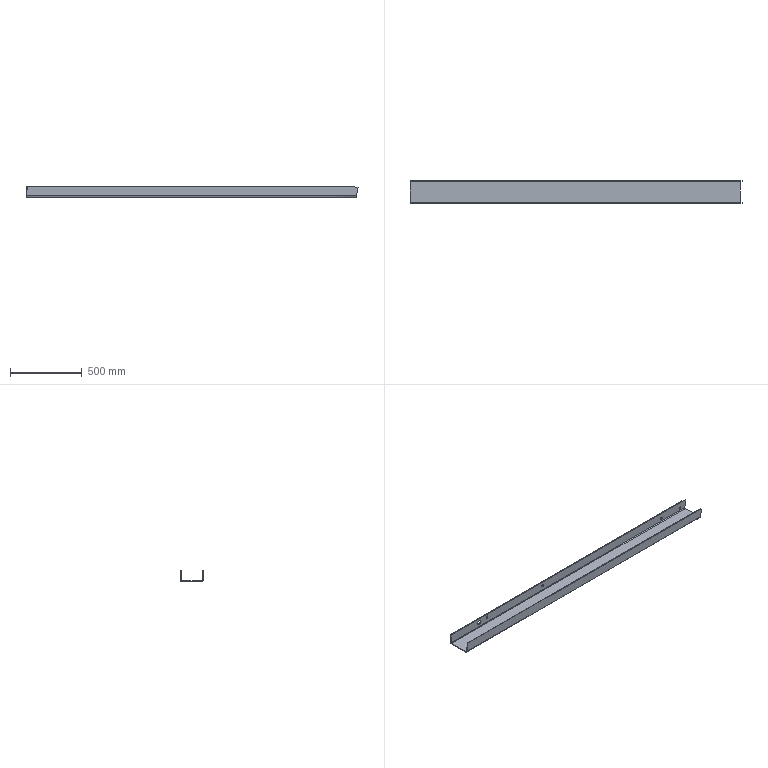Part | SolidWorks | features Split 4, Cut 2, 3DProfileFeature 1, FlatPattern 1, Fold 1, HoleWzd 1, SM3dBend 1, SMBaseFlange 1, SheetMetal 1, UnFold 1, WeldmentFeature 1 | 1 solid | 35 faces | box 2311 x 160 x 74.999 mm | volume 3368982 mm3 | plane 18 | cylinder 14 | spline 3 | commonest cylinder face diameters 18 x8 10 x2 20 x2 30 x2
STEP:
#1=CARTESIAN_POINT('',(-396.279,75.,50.082));
#2=VERTEX_POINT('',#1);
#3=CARTESIAN_POINT('',(-396.279,75.,32.082));
#4=VERTEX_POINT('',#3);
#5=CARTESIAN_POINT('',(-396.279,75.,41.082));
#6=DIRECTION('',(0.,-1.,0.));
#7=DIRECTION('',(0.,0.,-1.));
#8=AXIS2_PLACEMENT_3D('',#5,#6,#7);
#9=CIRCLE('',#8,9.);
#10=EDGE_CURVE('',#2,#4,#9,.T.);
#11=ORIENTED_EDGE('',*,*,#10,.T.);
#12=CARTESIAN_POINT('',(-396.279,80.,32.082));
#13=VERTEX_POINT('',#12);
#14=CARTESIAN_POINT('',(-396.279,80.,32.082));
#15=DIRECTION('',(0.,1.,0.));
#16=VECTOR('',#15,1000.);
#17=LINE('',#14,#16);
#18=EDGE_CURVE('',#4,#13,#17,.T.);
#19=ORIENTED_EDGE('',*,*,#18,.T.);
#20=CARTESIAN_POINT('',(-396.279,80.,50.082));
#21=VERTEX_POINT('',#20);
#22=CARTESIAN_POINT('',(-396.279,80.,41.082));
#23=DIRECTION('',(0.,1.,0.));
#24=DIRECTION('',(0.,0.,1.));
#25=AXIS2_PLACEMENT_3D('',#22,#23,#24);
#26=CIRCLE('',#25,9.);
#27=EDGE_CURVE('',#13,#21,#26,.T.);
#28=ORIENTED_EDGE('',*,*,#27,.T.);
#29=CARTESIAN_POINT('',(-396.279,80.,50.082));
#30=DIRECTION('',(0.,1.,0.));
#31=VECTOR('',#30,1000.);
#32=LINE('',#29,#31);
#33=EDGE_CURVE('',#2,#21,#32,.T.);
#34=ORIENTED_EDGE('',*,*,#33,.F.);
#35=EDGE_LOOP('',(#11,#19,#28,#34));
#36=FACE_OUTER_BOUND('',#35,.T.);
#37=CARTESIAN_POINT('',(-396.279,80.,41.082));
#38=DIRECTION('',(0.,1.,0.));
#39=DIRECTION('',(0.,0.,1.));
#40=AXIS2_PLACEMENT_3D('',#37,#38,#39);
#41=CYLINDRICAL_SURFACE('',#40,9.);
#42=ADVANCED_FACE('',(#36),#41,.F.);
#43=CARTESIAN_POINT('',(-945.843,75.,53.474));
#44=VERTEX_POINT('',#43);
#45=CARTESIAN_POINT('',(-945.843,75.,35.474));
#46=VERTEX_POINT('',#45);
#47=CARTESIAN_POINT('',(-945.843,75.,44.474));
#48=DIRECTION('',(0.,-1.,0.));
#49=DIRECTION('',(0.,0.,-1.));
#50=AXIS2_PLACEMENT_3D('',#47,#48,#49);
#51=CIRCLE('',#50,9.);
#52=EDGE_CURVE('',#44,#46,#51,.T.);
#53=ORIENTED_EDGE('',*,*,#52,.T.);
#54=CARTESIAN_POINT('',(-945.843,80.,35.474));
#55=VERTEX_POINT('',#54);
#56=CARTESIAN_POINT('',(-945.843,80.,35.474));
#57=DIRECTION('',(0.,1.,0.));
#58=VECTOR('',#57,1000.);
#59=LINE('',#56,#58);
#60=EDGE_CURVE('',#46,#55,#59,.T.);
#61=ORIENTED_EDGE('',*,*,#60,.T.);
#62=CARTESIAN_POINT('',(-945.843,80.,53.474));
#63=VERTEX_POINT('',#62);
#64=CARTESIAN_POINT('',(-945.843,80.,44.474));
#65=DIRECTION('',(0.,1.,0.));
#66=DIRECTION('',(0.,0.,1.));
#67=AXIS2_PLACEMENT_3D('',#64,#65,#66);
#68=CIRCLE('',#67,9.);
#69=EDGE_CURVE('',#55,#63,#68,.T.);
#70=ORIENTED_EDGE('',*,*,#69,.T.);
#71=CARTESIAN_POINT('',(-945.843,80.,53.474));
#72=DIRECTION('',(0.,1.,0.));
#73=VECTOR('',#72,1000.);
#74=LINE('',#71,#73);
#75=EDGE_CURVE('',#44,#63,#74,.T.);
#76=ORIENTED_EDGE('',*,*,#75,.F.);
#77=EDGE_LOOP('',(#53,#61,#70,#76));
#78=FACE_OUTER_BOUND('',#77,.T.);
#79=CARTESIAN_POINT('',(-945.843,80.,44.474));
#80=DIRECTION('',(0.,1.,0.));
#81=DIRECTION('',(0.,0.,1.));
#82=AXIS2_PLACEMENT_3D('',#79,#80,#81);
#83=CYLINDRICAL_SURFACE('',#82,9.);
#84=ADVANCED_FACE('',(#78),#83,.F.);
#85=CARTESIAN_POINT('',(772.235,75.,37.443));
#86=VERTEX_POINT('',#85);
#87=CARTESIAN_POINT('',(772.235,75.,19.443));
#88=VERTEX_POINT('',#87);
#89=CARTESIAN_POINT('',(772.235,75.,28.443));
#90=DIRECTION('',(0.,-1.,0.));
#91=DIRECTION('',(0.,0.,-1.));
#92=AXIS2_PLACEMENT_3D('',#89,#90,#91);
#93=CIRCLE('',#92,9.);
#94=EDGE_CURVE('',#86,#88,#93,.T.);
#95=ORIENTED_EDGE('',*,*,#94,.T.);
#96=CARTESIAN_POINT('',(772.235,80.,19.443));
#97=VERTEX_POINT('',#96);
#98=CARTESIAN_POINT('',(772.235,70.,19.443));
#99=DIRECTION('',(0.,1.,0.));
#100=VECTOR('',#99,1000.);
#101=LINE('',#98,#100);
#102=EDGE_CURVE('',#88,#97,#101,.T.);
#103=ORIENTED_EDGE('',*,*,#102,.T.);
#104=CARTESIAN_POINT('',(772.235,80.,37.443));
#105=VERTEX_POINT('',#104);
#106=CARTESIAN_POINT('',(772.235,80.,28.443));
#107=DIRECTION('',(0.,1.,0.));
#108=DIRECTION('',(0.,0.,1.));
#109=AXIS2_PLACEMENT_3D('',#106,#107,#108);
#110=CIRCLE('',#109,9.);
#111=EDGE_CURVE('',#97,#105,#110,.T.);
#112=ORIENTED_EDGE('',*,*,#111,.T.);
#113=CARTESIAN_POINT('',(772.235,70.,37.443));
#114=DIRECTION('',(0.,1.,0.));
#115=VECTOR('',#114,1000.);
#116=LINE('',#113,#115);
#117=EDGE_CURVE('',#86,#105,#116,.T.);
#118=ORIENTED_EDGE('',*,*,#117,.F.);
#119=EDGE_LOOP('',(#95,#103,#112,#118));
#120=FACE_OUTER_BOUND('',#119,.T.);
#121=CARTESIAN_POINT('',(772.235,70.,28.443));
#122=DIRECTION('',(0.,1.,0.));
#123=DIRECTION('',(0.,0.,1.));
#124=AXIS2_PLACEMENT_3D('',#121,#122,#123);
#125=CYLINDRICAL_SURFACE('',#124,9.);
#126=ADVANCED_FACE('',(#120),#125,.F.);
#127=CARTESIAN_POINT('',(953.893,75.,32.391));
#128=VERTEX_POINT('',#127);
#129=CARTESIAN_POINT('',(953.893,75.,14.391));
#130=VERTEX_POINT('',#129);
#131=CARTESIAN_POINT('',(953.893,75.,23.391));
#132=DIRECTION('',(0.,-1.,0.));
#133=DIRECTION('',(0.,0.,-1.));
#134=AXIS2_PLACEMENT_3D('',#131,#132,#133);
#135=CIRCLE('',#134,9.);
#136=EDGE_CURVE('',#128,#130,#135,.T.);
#137=ORIENTED_EDGE('',*,*,#136,.T.);
#138=CARTESIAN_POINT('',(953.893,80.,14.391));
#139=VERTEX_POINT('',#138);
#140=CARTESIAN_POINT('',(953.893,70.,14.391));
#141=DIRECTION('',(0.,1.,0.));
#142=VECTOR('',#141,1000.);
#143=LINE('',#140,#142);
#144=EDGE_CURVE('',#130,#139,#143,.T.);
#145=ORIENTED_EDGE('',*,*,#144,.T.);
#146=CARTESIAN_POINT('',(953.893,80.,32.391));
#147=VERTEX_POINT('',#146);
#148=CARTESIAN_POINT('',(953.893,80.,23.391));
#149=DIRECTION('',(0.,1.,0.));
#150=DIRECTION('',(0.,0.,1.));
#151=AXIS2_PLACEMENT_3D('',#148,#149,#150);
#152=CIRCLE('',#151,9.);
#153=EDGE_CURVE('',#139,#147,#152,.T.);
#154=ORIENTED_EDGE('',*,*,#153,.T.);
#155=CARTESIAN_POINT('',(953.893,70.,32.391));
#156=DIRECTION('',(0.,1.,0.));
#157=VECTOR('',#156,1000.);
#158=LINE('',#155,#157);
#159=EDGE_CURVE('',#128,#147,#158,.T.);
#160=ORIENTED_EDGE('',*,*,#159,.F.);
#161=EDGE_LOOP('',(#137,#145,#154,#160));
#162=FACE_OUTER_BOUND('',#161,.T.);
#163=CARTESIAN_POINT('',(953.893,70.,23.391));
#164=DIRECTION('',(0.,1.,0.));
#165=DIRECTION('',(0.,0.,1.));
#166=AXIS2_PLACEMENT_3D('',#163,#164,#165);
#167=CYLINDRICAL_SURFACE('',#166,9.);
#168=ADVANCED_FACE('',(#162),#167,.F.);
#169=CARTESIAN_POINT('',(-1024.117,75.,52.057));
#170=VERTEX_POINT('',#169);
#171=CARTESIAN_POINT('',(-1024.117,75.,22.057));
#172=VERTEX_POINT('',#171);
#173=CARTESIAN_POINT('',(-1024.117,75.,37.057));
#174=DIRECTION('',(0.,-1.,0.));
#175=DIRECTION('',(0.,0.,-1.));
#176=AXIS2_PLACEMENT_3D('',#173,#174,#175);
#177=CIRCLE('',#176,15.);
#178=EDGE_CURVE('',#170,#172,#177,.T.);
#179=ORIENTED_EDGE('',*,*,#178,.T.);
#180=CARTESIAN_POINT('',(-1024.117,80.,22.057));
#181=VERTEX_POINT('',#180);
#182=CARTESIAN_POINT('',(-1024.117,70.,22.057));
#183=DIRECTION('',(0.,1.,0.));
#184=VECTOR('',#183,1000.);
#185=LINE('',#182,#184);
#186=EDGE_CURVE('',#172,#181,#185,.T.);
#187=ORIENTED_EDGE('',*,*,#186,.T.);
#188=CARTESIAN_POINT('',(-1024.117,80.,52.057));
#189=VERTEX_POINT('',#188);
#190=CARTESIAN_POINT('',(-1024.117,80.,37.057));
#191=DIRECTION('',(0.,1.,0.));
#192=DIRECTION('',(0.,0.,1.));
#193=AXIS2_PLACEMENT_3D('',#190,#191,#192);
#194=CIRCLE('',#193,15.);
#195=EDGE_CURVE('',#181,#189,#194,.T.);
#196=ORIENTED_EDGE('',*,*,#195,.T.);
#197=CARTESIAN_POINT('',(-1024.117,70.,52.057));
#198=DIRECTION('',(0.,1.,0.));
#199=VECTOR('',#198,1000.);
#200=LINE('',#197,#199);
#201=EDGE_CURVE('',#170,#189,#200,.T.);
#202=ORIENTED_EDGE('',*,*,#201,.F.);
#203=EDGE_LOOP('',(#179,#187,#196,#202));
#204=FACE_OUTER_BOUND('',#203,.T.);
#205=CARTESIAN_POINT('',(-1024.117,70.,37.057));
#206=DIRECTION('',(0.,1.,0.));
#207=DIRECTION('',(0.,0.,1.));
#208=AXIS2_PLACEMENT_3D('',#205,#206,#207);
#209=CYLINDRICAL_SURFACE('',#208,15.);
#210=ADVANCED_FACE('',(#204),#209,.F.);
#211=CARTESIAN_POINT('',(-945.843,80.,44.474));
#212=DIRECTION('',(0.,1.,0.));
#213=DIRECTION('',(0.,0.,1.));
#214=AXIS2_PLACEMENT_3D('',#211,#212,#213);
#215=CIRCLE('',#214,9.);
#216=EDGE_CURVE('',#63,#55,#215,.T.);
#217=ORIENTED_EDGE('',*,*,#216,.F.);
#218=ORIENTED_EDGE('',*,*,#69,.F.);
#219=EDGE_LOOP('',(#217,#218));
#220=FACE_BOUND('',#219,.T.);
#221=CARTESIAN_POINT('',(772.235,80.,28.443));
#222=DIRECTION('',(0.,1.,0.));
#223=DIRECTION('',(0.,0.,1.));
#224=AXIS2_PLACEMENT_3D('',#221,#222,#223);
#225=CIRCLE('',#224,9.);
#226=EDGE_CURVE('',#105,#97,#225,.T.);
#227=ORIENTED_EDGE('',*,*,#226,.F.);
#228=ORIENTED_EDGE('',*,*,#111,.F.);
#229=EDGE_LOOP('',(#227,#228));
#230=FACE_BOUND('',#229,.T.);
#231=CARTESIAN_POINT('',(953.893,80.,23.391));
#232=DIRECTION('',(0.,1.,0.));
#233=DIRECTION('',(0.,0.,1.));
#234=AXIS2_PLACEMENT_3D('',#231,#232,#233);
#235=CIRCLE('',#234,9.);
#236=EDGE_CURVE('',#147,#139,#235,.T.);
#237=ORIENTED_EDGE('',*,*,#236,.F.);
#238=ORIENTED_EDGE('',*,*,#153,.F.);
#239=EDGE_LOOP('',(#237,#238));
#240=FACE_BOUND('',#239,.T.);
#241=CARTESIAN_POINT('',(-1024.117,80.,37.057));
#242=DIRECTION('',(0.,1.,0.));
#243=DIRECTION('',(0.,0.,1.));
#244=AXIS2_PLACEMENT_3D('',#241,#242,#243);
#245=CIRCLE('',#244,15.);
#246=EDGE_CURVE('',#189,#181,#245,.T.);
#247=ORIENTED_EDGE('',*,*,#246,.F.);
#248=ORIENTED_EDGE('',*,*,#195,.F.);
#249=EDGE_LOOP('',(#247,#248));
#250=FACE_BOUND('',#249,.T.);
#251=CARTESIAN_POINT('',(-1299.9,80.,69.999));
#252=VERTEX_POINT('',#251);
#253=CARTESIAN_POINT('',(-1299.9,80.,5.));
#254=VERTEX_POINT('',#253);
#255=CARTESIAN_POINT('',(-1299.9,80.,-76.781));
#256=DIRECTION('',(0.,0.,-1.));
#257=VECTOR('',#256,1000.);
#258=LINE('',#255,#257);
#259=EDGE_CURVE('',#252,#254,#258,.T.);
#260=ORIENTED_EDGE('',*,*,#259,.F.);
#261=CARTESIAN_POINT('',(978.319,80.,69.999));
#262=VERTEX_POINT('',#261);
#263=CARTESIAN_POINT('',(-1300.,80.,69.999));
#264=DIRECTION('',(-1.,0.,0.));
#265=VECTOR('',#264,1000.);
#266=LINE('',#263,#265);
#267=EDGE_CURVE('',#262,#252,#266,.T.);
#268=ORIENTED_EDGE('',*,*,#267,.F.);
#269=CARTESIAN_POINT('',(1011.459,80.,64.453));
#270=VERTEX_POINT('',#269);
#271=CARTESIAN_POINT('',(50.544,80.,225.255));
#272=DIRECTION('',(-0.9863,0.,0.165));
#273=VECTOR('',#272,1000.);
#274=LINE('',#271,#273);
#275=EDGE_CURVE('',#270,#262,#274,.T.);
#276=ORIENTED_EDGE('',*,*,#275,.F.);
#277=CARTESIAN_POINT('',(1001.51,80.,5.));
#278=VERTEX_POINT('',#277);
#279=CARTESIAN_POINT('',(960.916,80.,-237.583));
#280=DIRECTION('',(-0.165,0.,-0.9863));
#281=VECTOR('',#280,1000.);
#282=LINE('',#279,#281);
#283=EDGE_CURVE('',#270,#278,#282,.T.);
#284=ORIENTED_EDGE('',*,*,#283,.T.);
#285=CARTESIAN_POINT('',(-1299.9,80.,5.));
#286=CARTESIAN_POINT('',(-532.763,80.,5.));
#287=CARTESIAN_POINT('',(234.373,80.,5.));
#288=CARTESIAN_POINT('',(1001.51,80.,5.));
#289=B_SPLINE_CURVE_WITH_KNOTS('',3,(#285,#286,#287,#288),.UNSPECIFIED.,.F.,.F.,(4,4),(0.,1.),.UNSPECIFIED.);
#290=EDGE_CURVE('',#254,#278,#289,.T.);
#291=ORIENTED_EDGE('',*,*,#290,.F.);
#292=EDGE_LOOP('',(#260,#268,#276,#284,#291));
#293=FACE_OUTER_BOUND('',#292,.T.);
#294=CARTESIAN_POINT('',(-396.279,80.,41.082));
#295=DIRECTION('',(0.,1.,0.));
#296=DIRECTION('',(0.,0.,1.));
#297=AXIS2_PLACEMENT_3D('',#294,#295,#296);
#298=CIRCLE('',#297,9.);
#299=EDGE_CURVE('',#21,#13,#298,.T.);
#300=ORIENTED_EDGE('',*,*,#299,.F.);
#301=ORIENTED_EDGE('',*,*,#27,.F.);
#302=EDGE_LOOP('',(#300,#301));
#303=FACE_BOUND('',#302,.T.);
#304=CARTESIAN_POINT('',(0.,80.,-76.781));
#305=DIRECTION('',(0.,-1.,0.));
#306=DIRECTION('',(1.,0.,0.));
#307=AXIS2_PLACEMENT_3D('',#304,#305,#306);
#308=PLANE('',#307);
#309=ADVANCED_FACE('',(#220,#230,#240,#250,#293,#303),#308,.F.);
#310=CARTESIAN_POINT('',(1000.673,70.,0.));
#311=VERTEX_POINT('',#310);
#312=CARTESIAN_POINT('',(-1299.9,70.,0.));
#313=VERTEX_POINT('',#312);
#314=CARTESIAN_POINT('',(1000.673,70.,0.));
#315=CARTESIAN_POINT('',(233.816,70.,0.));
#316=CARTESIAN_POINT('',(-533.042,70.,0.));
#317=CARTESIAN_POINT('',(-1299.9,70.,0.));
#318=B_SPLINE_CURVE_WITH_KNOTS('',3,(#314,#315,#316,#317),.UNSPECIFIED.,.F.,.F.,(4,4),(0.,1.),.UNSPECIFIED.);
#319=EDGE_CURVE('',#311,#313,#318,.T.);
#320=ORIENTED_EDGE('',*,*,#319,.T.);
#321=CARTESIAN_POINT('',(-1299.9,-70.,0.));
#322=VERTEX_POINT('',#321);
#323=CARTESIAN_POINT('',(-1299.9,0.,0.));
#324=DIRECTION('',(0.,-1.,0.));
#325=VECTOR('',#324,1000.);
#326=LINE('',#323,#325);
#327=EDGE_CURVE('',#313,#322,#326,.T.);
#328=ORIENTED_EDGE('',*,*,#327,.T.);
#329=CARTESIAN_POINT('',(1000.673,-70.,0.));
#330=VERTEX_POINT('',#329);
#331=CARTESIAN_POINT('',(-1299.9,-70.,0.));
#332=CARTESIAN_POINT('',(-533.042,-70.,0.));
#333=CARTESIAN_POINT('',(233.816,-70.,0.));
#334=CARTESIAN_POINT('',(1000.673,-70.,0.));
#335=B_SPLINE_CURVE_WITH_KNOTS('',3,(#331,#332,#333,#334),.UNSPECIFIED.,.F.,.F.,(4,4),(0.,1.),.UNSPECIFIED.);
#336=EDGE_CURVE('',#322,#330,#335,.T.);
#337=ORIENTED_EDGE('',*,*,#336,.T.);
#338=CARTESIAN_POINT('',(1000.673,0.,0.));
#339=DIRECTION('',(0.,-1.,0.));
#340=VECTOR('',#339,1000.);
#341=LINE('',#338,#340);
#342=EDGE_CURVE('',#311,#330,#341,.T.);
#343=ORIENTED_EDGE('',*,*,#342,.F.);
#344=EDGE_LOOP('',(#320,#328,#337,#343));
#345=FACE_OUTER_BOUND('',#344,.T.);
#346=CARTESIAN_POINT('',(0.,0.,0.));
#347=DIRECTION('',(0.,0.,1.));
#348=DIRECTION('',(1.,0.,0.));
#349=AXIS2_PLACEMENT_3D('',#346,#347,#348);
#350=PLANE('',#349);
#351=ADVANCED_FACE('',(#345),#350,.T.);
#352=CARTESIAN_POINT('',(999.837,-70.,-5.));
#353=VERTEX_POINT('',#352);
#354=CARTESIAN_POINT('',(999.837,-70.,-5.));
#355=CARTESIAN_POINT('',(1000.673,-70.,0.));
#356=B_SPLINE_CURVE_WITH_KNOTS('',1,(#354,#355),.UNSPECIFIED.,.F.,.F.,(2,2),(0.,1.),.UNSPECIFIED.);
#357=EDGE_CURVE('',#353,#330,#356,.T.);
#358=ORIENTED_EDGE('',*,*,#357,.F.);
#359=CARTESIAN_POINT('',(999.837,70.,-5.));
#360=VERTEX_POINT('',#359);
#361=CARTESIAN_POINT('',(999.837,0.,-5.));
#362=DIRECTION('',(0.,-1.,0.));
#363=VECTOR('',#362,1000.);
#364=LINE('',#361,#363);
#365=EDGE_CURVE('',#360,#353,#364,.T.);
#366=ORIENTED_EDGE('',*,*,#365,.F.);
#367=CARTESIAN_POINT('',(1000.673,70.,0.));
#368=CARTESIAN_POINT('',(999.837,70.,-5.));
#369=B_SPLINE_CURVE_WITH_KNOTS('',1,(#367,#368),.UNSPECIFIED.,.F.,.F.,(2,2),(0.,1.),.UNSPECIFIED.);
#370=EDGE_CURVE('',#311,#360,#369,.T.);
#371=ORIENTED_EDGE('',*,*,#370,.F.);
#372=ORIENTED_EDGE('',*,*,#342,.T.);
#373=EDGE_LOOP('',(#358,#366,#371,#372));
#374=FACE_OUTER_BOUND('',#373,.T.);
#375=CARTESIAN_POINT('',(973.414,0.,-162.894));
#376=DIRECTION('',(-0.9863,0.,0.165));
#377=DIRECTION('',(0.165,0.,0.9863));
#378=AXIS2_PLACEMENT_3D('',#375,#376,#377);
#379=PLANE('',#378);
#380=ADVANCED_FACE('',(#374),#379,.F.);
#381=CARTESIAN_POINT('',(-1299.9,70.,-5.));
#382=VERTEX_POINT('',#381);
#383=CARTESIAN_POINT('',(-1299.9,-70.,-5.));
#384=VERTEX_POINT('',#383);
#385=CARTESIAN_POINT('',(-1299.9,0.,-5.));
#386=DIRECTION('',(0.,-1.,0.));
#387=VECTOR('',#386,1000.);
#388=LINE('',#385,#387);
#389=EDGE_CURVE('',#382,#384,#388,.T.);
#390=ORIENTED_EDGE('',*,*,#389,.F.);
#391=CARTESIAN_POINT('',(999.837,70.,-5.));
#392=CARTESIAN_POINT('',(233.258,70.,-5.));
#393=CARTESIAN_POINT('',(-533.321,70.,-5.));
#394=CARTESIAN_POINT('',(-1299.9,70.,-5.));
#395=B_SPLINE_CURVE_WITH_KNOTS('',3,(#391,#392,#393,#394),.UNSPECIFIED.,.F.,.F.,(4,4),(0.,1.),.UNSPECIFIED.);
#396=EDGE_CURVE('',#360,#382,#395,.T.);
#397=ORIENTED_EDGE('',*,*,#396,.F.);
#398=ORIENTED_EDGE('',*,*,#365,.T.);
#399=CARTESIAN_POINT('',(-1299.9,-70.,-5.));
#400=CARTESIAN_POINT('',(-533.321,-70.,-5.));
#401=CARTESIAN_POINT('',(233.258,-70.,-5.));
#402=CARTESIAN_POINT('',(999.837,-70.,-5.));
#403=B_SPLINE_CURVE_WITH_KNOTS('',3,(#399,#400,#401,#402),.UNSPECIFIED.,.F.,.F.,(4,4),(0.,1.),.UNSPECIFIED.);
#404=EDGE_CURVE('',#384,#353,#403,.T.);
#405=ORIENTED_EDGE('',*,*,#404,.F.);
#406=EDGE_LOOP('',(#390,#397,#398,#405));
#407=FACE_OUTER_BOUND('',#406,.T.);
#408=CARTESIAN_POINT('',(0.,0.,-5.));
#409=DIRECTION('',(0.,0.,1.));
#410=DIRECTION('',(1.,0.,0.));
#411=AXIS2_PLACEMENT_3D('',#408,#409,#410);
#412=PLANE('',#411);
#413=ADVANCED_FACE('',(#407),#412,.F.);
#414=CARTESIAN_POINT('',(-1299.9,-70.,0.));
#415=CARTESIAN_POINT('',(-1299.9,-70.,-1.667));
#416=CARTESIAN_POINT('',(-1299.9,-70.,-3.333));
#417=CARTESIAN_POINT('',(-1299.9,-70.,-5.));
#418=B_SPLINE_CURVE_WITH_KNOTS('',3,(#414,#415,#416,#417),.UNSPECIFIED.,.F.,.F.,(4,4),(0.,1.),.UNSPECIFIED.);
#419=EDGE_CURVE('',#322,#384,#418,.T.);
#420=ORIENTED_EDGE('',*,*,#419,.F.);
#421=ORIENTED_EDGE('',*,*,#327,.F.);
#422=CARTESIAN_POINT('',(-1299.9,70.,0.));
#423=CARTESIAN_POINT('',(-1299.9,70.,-1.667));
#424=CARTESIAN_POINT('',(-1299.9,70.,-3.333));
#425=CARTESIAN_POINT('',(-1299.9,70.,-5.));
#426=B_SPLINE_CURVE_WITH_KNOTS('',3,(#422,#423,#424,#425),.UNSPECIFIED.,.F.,.F.,(4,4),(0.,1.),.UNSPECIFIED.);
#427=EDGE_CURVE('',#313,#382,#426,.T.);
#428=ORIENTED_EDGE('',*,*,#427,.T.);
#429=ORIENTED_EDGE('',*,*,#389,.T.);
#430=EDGE_LOOP('',(#420,#421,#428,#429));
#431=FACE_OUTER_BOUND('',#430,.T.);
#432=CARTESIAN_POINT('',(-1299.9,0.,0.));
#433=DIRECTION('',(-1.,0.,0.));
#434=DIRECTION('',(0.,0.,1.));
#435=AXIS2_PLACEMENT_3D('',#432,#433,#434);
#436=PLANE('',#435);
#437=ADVANCED_FACE('',(#431),#436,.T.);
#438=ORIENTED_EDGE('',*,*,#427,.F.);
#439=CARTESIAN_POINT('',(-1299.9,75.,5.));
#440=VERTEX_POINT('',#439);
#441=CARTESIAN_POINT('',(-1299.9,70.,5.));
#442=DIRECTION('',(1.,0.,0.));
#443=DIRECTION('',(0.,0.,-1.));
#444=AXIS2_PLACEMENT_3D('',#441,#442,#443);
#445=CIRCLE('',#444,5.);
#446=EDGE_CURVE('',#313,#440,#445,.T.);
#447=ORIENTED_EDGE('',*,*,#446,.T.);
#448=CARTESIAN_POINT('',(-1299.9,75.,5.));
#449=CARTESIAN_POINT('',(-1299.9,76.667,5.));
#450=CARTESIAN_POINT('',(-1299.9,78.333,5.));
#451=CARTESIAN_POINT('',(-1299.9,80.,5.));
#452=B_SPLINE_CURVE_WITH_KNOTS('',3,(#448,#449,#450,#451),.UNSPECIFIED.,.F.,.F.,(4,4),(0.,1.),.UNSPECIFIED.);
#453=EDGE_CURVE('',#440,#254,#452,.T.);
#454=ORIENTED_EDGE('',*,*,#453,.T.);
#455=CARTESIAN_POINT('',(-1299.9,70.,5.));
#456=DIRECTION('',(1.,0.,0.));
#457=DIRECTION('',(0.,0.,-1.));
#458=AXIS2_PLACEMENT_3D('',#455,#456,#457);
#459=CIRCLE('',#458,10.);
#460=EDGE_CURVE('',#382,#254,#459,.T.);
#461=ORIENTED_EDGE('',*,*,#460,.F.);
#462=EDGE_LOOP('',(#438,#447,#454,#461));
#463=FACE_OUTER_BOUND('',#462,.T.);
#464=CARTESIAN_POINT('',(-1299.9,70.,5.));
#465=DIRECTION('',(-1.,0.,0.));
#466=DIRECTION('',(0.,0.,1.));
#467=AXIS2_PLACEMENT_3D('',#464,#465,#466);
#468=PLANE('',#467);
#469=ADVANCED_FACE('',(#463),#468,.T.);
#470=CARTESIAN_POINT('',(1001.51,80.,5.));
#471=CARTESIAN_POINT('',(1001.367,80.,4.143));
#472=CARTESIAN_POINT('',(1001.242,79.891,3.392));
#473=CARTESIAN_POINT('',(1001.083,79.672,2.439));
#474=CARTESIAN_POINT('',(1001.034,79.589,2.15));
#475=CARTESIAN_POINT('',(1000.968,79.461,1.758));
#476=CARTESIAN_POINT('',(1000.948,79.417,1.634));
#477=CARTESIAN_POINT('',(1000.918,79.352,1.459));
#478=CARTESIAN_POINT('',(1000.904,79.32,1.374));
#479=CARTESIAN_POINT('',(1000.888,79.282,1.279));
#480=CARTESIAN_POINT('',(1000.88,79.263,1.233));
#481=CARTESIAN_POINT('',(1000.877,79.254,1.21));
#482=CARTESIAN_POINT('',(1000.875,79.25,1.2));
#483=CARTESIAN_POINT('',(1000.874,79.247,1.194));
#484=CARTESIAN_POINT('',(1000.874,79.247,1.193));
#485=CARTESIAN_POINT('',(1000.762,78.972,0.5253));
#486=CARTESIAN_POINT('',(1000.662,78.64,-0.07712));
#487=CARTESIAN_POINT('',(1000.526,78.091,-0.8862));
#488=CARTESIAN_POINT('',(1000.483,77.899,-1.14));
#489=CARTESIAN_POINT('',(1000.423,77.602,-1.498));
#490=CARTESIAN_POINT('',(1000.404,77.502,-1.614));
#491=CARTESIAN_POINT('',(1000.376,77.35,-1.781));
#492=CARTESIAN_POINT('',(1000.362,77.273,-1.864));
#493=CARTESIAN_POINT('',(1000.346,77.183,-1.957));
#494=CARTESIAN_POINT('',(1000.338,77.138,-2.003));
#495=CARTESIAN_POINT('',(1000.335,77.119,-2.023));
#496=CARTESIAN_POINT('',(1000.333,77.106,-2.036));
#497=CARTESIAN_POINT('',(1000.332,77.101,-2.041));
#498=CARTESIAN_POINT('',(1000.248,76.606,-2.54));
#499=CARTESIAN_POINT('',(1000.177,76.08,-2.966));
#500=CARTESIAN_POINT('',(1000.086,75.261,-3.51));
#501=CARTESIAN_POINT('',(1000.058,74.983,-3.676));
#502=CARTESIAN_POINT('',(1000.02,74.561,-3.901));
#503=CARTESIAN_POINT('',(1000.003,74.349,-4.007));
#504=CARTESIAN_POINT('',(999.986,74.135,-4.105));
#505=CARTESIAN_POINT('',(999.976,73.993,-4.169));
#506=CARTESIAN_POINT('',(999.971,73.923,-4.199));
#507=CARTESIAN_POINT('',(999.885,72.673,-4.72));
#508=CARTESIAN_POINT('',(999.842,71.36,-5.));
#509=CARTESIAN_POINT('',(999.837,70.,-5.));
#510=B_SPLINE_CURVE_WITH_KNOTS('',3,(#470,#471,#472,#473,#474,#475,#476,#477,#478,#479,#480,#481,#482,#483,#484,#485,#486,#487,#488,#489,#490,#491,#492,#493,#494,#495,#496,#497,#498,#499,#500,#501,#502,#503,#504,#505,#506,#507,#508,#509),.UNSPECIFIED.,.F.,.F.,(4,2,2,2,1,1,1,1,2,2,2,2,2,1,1,1,2,2,2,2,1,2,2,4),(0.,0.125,0.1875,0.2188,0.2344,0.2422,0.2461,0.248,0.249,0.25,0.375,0.4375,0.4688,0.4844,0.4922,0.4961,0.498,0.5,0.625,0.6875,0.7188,0.7344,0.75,1.),.UNSPECIFIED.);
#511=EDGE_CURVE('',#278,#360,#510,.T.);
#512=ORIENTED_EDGE('',*,*,#511,.T.);
#513=ORIENTED_EDGE('',*,*,#396,.T.);
#514=ORIENTED_EDGE('',*,*,#460,.T.);
#515=ORIENTED_EDGE('',*,*,#290,.T.);
#516=EDGE_LOOP('',(#512,#513,#514,#515));
#517=FACE_OUTER_BOUND('',#516,.T.);
#518=CARTESIAN_POINT('',(-2451.528,70.,5.));
#519=DIRECTION('',(1.,0.,0.));
#520=DIRECTION('',(0.,0.,-1.));
#521=AXIS2_PLACEMENT_3D('',#518,#519,#520);
#522=CYLINDRICAL_SURFACE('',#521,10.);
#523=ADVANCED_FACE('',(#517),#522,.T.);
#524=CARTESIAN_POINT('',(1001.51,75.,5.));
#525=VERTEX_POINT('',#524);
#526=CARTESIAN_POINT('',(-1299.9,75.,5.));
#527=CARTESIAN_POINT('',(-532.763,75.,5.));
#528=CARTESIAN_POINT('',(234.373,75.,5.));
#529=CARTESIAN_POINT('',(1001.51,75.,5.));
#530=B_SPLINE_CURVE_WITH_KNOTS('',3,(#526,#527,#528,#529),.UNSPECIFIED.,.F.,.F.,(4,4),(0.,1.),.UNSPECIFIED.);
#531=EDGE_CURVE('',#440,#525,#530,.T.);
#532=ORIENTED_EDGE('',*,*,#531,.F.);
#533=ORIENTED_EDGE('',*,*,#446,.F.);
#534=ORIENTED_EDGE('',*,*,#319,.F.);
#535=CARTESIAN_POINT('',(1001.51,75.,5.));
#536=CARTESIAN_POINT('',(1001.396,75.,4.351));
#537=CARTESIAN_POINT('',(1001.18,74.744,3.051));
#538=CARTESIAN_POINT('',(1000.906,73.642,1.386));
#539=CARTESIAN_POINT('',(1000.719,71.977,0.2641));
#540=CARTESIAN_POINT('',(1000.68,70.659,0.000000132));
#541=CARTESIAN_POINT('',(1000.673,70.,0.));
#542=B_SPLINE_CURVE_WITH_KNOTS('',3,(#535,#536,#537,#538,#539,#540,#541),.UNSPECIFIED.,.F.,.F.,(4,1,1,1,4),(0.,0.25,0.5,0.75,1.),.UNSPECIFIED.);
#543=EDGE_CURVE('',#525,#311,#542,.T.);
#544=ORIENTED_EDGE('',*,*,#543,.F.);
#545=EDGE_LOOP('',(#532,#533,#534,#544));
#546=FACE_OUTER_BOUND('',#545,.T.);
#547=CARTESIAN_POINT('',(-2451.528,70.,5.));
#548=DIRECTION('',(1.,0.,0.));
#549=DIRECTION('',(0.,0.,-1.));
#550=AXIS2_PLACEMENT_3D('',#547,#548,#549);
#551=CYLINDRICAL_SURFACE('',#550,5.);
#552=ADVANCED_FACE('',(#546),#551,.F.);
#553=ORIENTED_EDGE('',*,*,#511,.F.);
#554=CARTESIAN_POINT('',(1001.51,80.,5.));
#555=CARTESIAN_POINT('',(1001.51,75.,5.));
#556=B_SPLINE_CURVE_WITH_KNOTS('',1,(#554,#555),.UNSPECIFIED.,.F.,.F.,(2,2),(0.,1.),.UNSPECIFIED.);
#557=EDGE_CURVE('',#278,#525,#556,.T.);
#558=ORIENTED_EDGE('',*,*,#557,.T.);
#559=ORIENTED_EDGE('',*,*,#543,.T.);
#560=ORIENTED_EDGE('',*,*,#370,.T.);
#561=EDGE_LOOP('',(#553,#558,#559,#560));
#562=FACE_OUTER_BOUND('',#561,.T.);
#563=CARTESIAN_POINT('',(1001.51,80.,5.));
#564=CARTESIAN_POINT('',(1001.51,75.,5.));
#565=CARTESIAN_POINT('',(1001.293,80.,3.7));
#566=CARTESIAN_POINT('',(1001.396,75.,4.351));
#567=CARTESIAN_POINT('',(1000.858,79.488,1.1));
#568=CARTESIAN_POINT('',(1001.18,74.744,3.051));
#569=CARTESIAN_POINT('',(1000.301,77.283,-2.227));
#570=CARTESIAN_POINT('',(1000.906,73.642,1.386));
#571=CARTESIAN_POINT('',(999.923,73.954,-4.472));
#572=CARTESIAN_POINT('',(1000.719,71.977,0.2641));
#573=CARTESIAN_POINT('',(999.842,71.318,-5.));
#574=CARTESIAN_POINT('',(1000.68,70.659,0.000000132));
#575=CARTESIAN_POINT('',(999.837,70.,-5.));
#576=CARTESIAN_POINT('',(1000.673,70.,0.));
#577=B_SPLINE_SURFACE_WITH_KNOTS('',3,1,((#563,#564),(#565,#566),(#567,#568),(#569,#570),(#571,#572),(#573,#574),(#575,#576)),.UNSPECIFIED.,.F.,.F.,.F.,(4,1,1,1,4),(2,2),(0.,0.25,0.5,0.75,1.),(0.,1.),.UNSPECIFIED.);
#578=ADVANCED_FACE('',(#562),#577,.F.);
#579=CARTESIAN_POINT('',(1011.459,75.,64.453));
#580=VERTEX_POINT('',#579);
#581=CARTESIAN_POINT('',(1011.459,-0.000000004,64.453));
#582=DIRECTION('',(0.,1.,0.));
#583=VECTOR('',#582,1000.);
#584=LINE('',#581,#583);
#585=EDGE_CURVE('',#580,#270,#584,.T.);
#586=ORIENTED_EDGE('',*,*,#585,.T.);
#587=ORIENTED_EDGE('',*,*,#275,.T.);
#588=CARTESIAN_POINT('',(978.319,75.,69.999));
#589=VERTEX_POINT('',#588);
#590=CARTESIAN_POINT('',(978.319,80.,69.999));
#591=DIRECTION('',(0.,1.,0.));
#592=VECTOR('',#591,1000.);
#593=LINE('',#590,#592);
#594=EDGE_CURVE('',#589,#262,#593,.T.);
#595=ORIENTED_EDGE('',*,*,#594,.F.);
#596=CARTESIAN_POINT('',(50.544,75.,225.255));
#597=DIRECTION('',(-0.9863,0.,0.165));
#598=VECTOR('',#597,1000.);
#599=LINE('',#596,#598);
#600=EDGE_CURVE('',#580,#589,#599,.T.);
#601=ORIENTED_EDGE('',*,*,#600,.F.);
#602=EDGE_LOOP('',(#586,#587,#595,#601));
#603=FACE_OUTER_BOUND('',#602,.T.);
#604=CARTESIAN_POINT('',(93.369,-0.0004862,218.089));
#605=DIRECTION('',(0.165,0.,0.9863));
#606=DIRECTION('',(0.9863,0.,-0.165));
#607=AXIS2_PLACEMENT_3D('',#604,#605,#606);
#608=PLANE('',#607);
#609=ADVANCED_FACE('',(#603),#608,.T.);
#610=ORIENTED_EDGE('',*,*,#267,.T.);
#611=CARTESIAN_POINT('',(-1299.9,75.,69.999));
#612=VERTEX_POINT('',#611);
#613=CARTESIAN_POINT('',(-1299.9,80.,69.999));
#614=DIRECTION('',(0.,-1.,0.));
#615=VECTOR('',#614,1000.);
#616=LINE('',#613,#615);
#617=EDGE_CURVE('',#252,#612,#616,.T.);
#618=ORIENTED_EDGE('',*,*,#617,.T.);
#619=CARTESIAN_POINT('',(-1300.,75.,69.999));
#620=DIRECTION('',(-1.,0.,0.));
#621=VECTOR('',#620,1000.);
#622=LINE('',#619,#621);
#623=EDGE_CURVE('',#589,#612,#622,.T.);
#624=ORIENTED_EDGE('',*,*,#623,.F.);
#625=ORIENTED_EDGE('',*,*,#594,.T.);
#626=EDGE_LOOP('',(#610,#618,#624,#625));
#627=FACE_OUTER_BOUND('',#626,.T.);
#628=CARTESIAN_POINT('',(-1300.,80.,69.999));
#629=DIRECTION('',(0.,0.,1.));
#630=DIRECTION('',(0.,-1.,0.));
#631=AXIS2_PLACEMENT_3D('',#628,#629,#630);
#632=PLANE('',#631);
#633=ADVANCED_FACE('',(#627),#632,.T.);
#634=ORIENTED_EDGE('',*,*,#186,.F.);
#635=CARTESIAN_POINT('',(-1024.117,75.,37.057));
#636=DIRECTION('',(0.,-1.,0.));
#637=DIRECTION('',(0.,0.,-1.));
#638=AXIS2_PLACEMENT_3D('',#635,#636,#637);
#639=CIRCLE('',#638,15.);
#640=EDGE_CURVE('',#172,#170,#639,.T.);
#641=ORIENTED_EDGE('',*,*,#640,.T.);
#642=ORIENTED_EDGE('',*,*,#201,.T.);
#643=ORIENTED_EDGE('',*,*,#246,.T.);
#644=EDGE_LOOP('',(#634,#641,#642,#643));
#645=FACE_OUTER_BOUND('',#644,.T.);
#646=CARTESIAN_POINT('',(-1024.117,70.,37.057));
#647=DIRECTION('',(0.,1.,0.));
#648=DIRECTION('',(0.,0.,1.));
#649=AXIS2_PLACEMENT_3D('',#646,#647,#648);
#650=CYLINDRICAL_SURFACE('',#649,15.);
#651=ADVANCED_FACE('',(#645),#650,.F.);
#652=ORIENTED_EDGE('',*,*,#453,.F.);
#653=CARTESIAN_POINT('',(-1299.9,75.,-76.781));
#654=DIRECTION('',(0.,0.,-1.));
#655=VECTOR('',#654,1000.);
#656=LINE('',#653,#655);
#657=EDGE_CURVE('',#612,#440,#656,.T.);
#658=ORIENTED_EDGE('',*,*,#657,.F.);
#659=ORIENTED_EDGE('',*,*,#617,.F.);
#660=ORIENTED_EDGE('',*,*,#259,.T.);
#661=EDGE_LOOP('',(#652,#658,#659,#660));
#662=FACE_OUTER_BOUND('',#661,.T.);
#663=CARTESIAN_POINT('',(-1299.9,-0.000000004,0.000000004));
#664=DIRECTION('',(-1.,0.,0.));
#665=DIRECTION('',(0.,0.,1.));
#666=AXIS2_PLACEMENT_3D('',#663,#664,#665);
#667=PLANE('',#666);
#668=ADVANCED_FACE('',(#662),#667,.T.);
#669=ORIENTED_EDGE('',*,*,#10,.F.);
#670=CARTESIAN_POINT('',(-396.279,75.,41.082));
#671=DIRECTION('',(0.,-1.,0.));
#672=DIRECTION('',(0.,0.,-1.));
#673=AXIS2_PLACEMENT_3D('',#670,#671,#672);
#674=CIRCLE('',#673,9.);
#675=EDGE_CURVE('',#4,#2,#674,.T.);
#676=ORIENTED_EDGE('',*,*,#675,.F.);
#677=EDGE_LOOP('',(#669,#676));
#678=FACE_BOUND('',#677,.T.);
#679=ORIENTED_EDGE('',*,*,#52,.F.);
#680=CARTESIAN_POINT('',(-945.843,75.,44.474));
#681=DIRECTION('',(0.,-1.,0.));
#682=DIRECTION('',(0.,0.,-1.));
#683=AXIS2_PLACEMENT_3D('',#680,#681,#682);
#684=CIRCLE('',#683,9.);
#685=EDGE_CURVE('',#46,#44,#684,.T.);
#686=ORIENTED_EDGE('',*,*,#685,.F.);
#687=EDGE_LOOP('',(#679,#686));
#688=FACE_BOUND('',#687,.T.);
#689=ORIENTED_EDGE('',*,*,#94,.F.);
#690=CARTESIAN_POINT('',(772.235,75.,28.443));
#691=DIRECTION('',(0.,-1.,0.));
#692=DIRECTION('',(0.,0.,-1.));
#693=AXIS2_PLACEMENT_3D('',#690,#691,#692);
#694=CIRCLE('',#693,9.);
#695=EDGE_CURVE('',#88,#86,#694,.T.);
#696=ORIENTED_EDGE('',*,*,#695,.F.);
#697=EDGE_LOOP('',(#689,#696));
#698=FACE_BOUND('',#697,.T.);
#699=ORIENTED_EDGE('',*,*,#136,.F.);
#700=CARTESIAN_POINT('',(953.893,75.,23.391));
#701=DIRECTION('',(0.,-1.,0.));
#702=DIRECTION('',(0.,0.,-1.));
#703=AXIS2_PLACEMENT_3D('',#700,#701,#702);
#704=CIRCLE('',#703,9.);
#705=EDGE_CURVE('',#130,#128,#704,.T.);
#706=ORIENTED_EDGE('',*,*,#705,.F.);
#707=EDGE_LOOP('',(#699,#706));
#708=FACE_BOUND('',#707,.T.);
#709=ORIENTED_EDGE('',*,*,#178,.F.);
#710=ORIENTED_EDGE('',*,*,#640,.F.);
#711=EDGE_LOOP('',(#709,#710));
#712=FACE_BOUND('',#711,.T.);
#713=ORIENTED_EDGE('',*,*,#623,.T.);
#714=ORIENTED_EDGE('',*,*,#657,.T.);
#715=ORIENTED_EDGE('',*,*,#531,.T.);
#716=CARTESIAN_POINT('',(960.916,75.,-237.583));
#717=DIRECTION('',(-0.165,0.,-0.9863));
#718=VECTOR('',#717,1000.);
#719=LINE('',#716,#718);
#720=EDGE_CURVE('',#580,#525,#719,.T.);
#721=ORIENTED_EDGE('',*,*,#720,.F.);
#722=ORIENTED_EDGE('',*,*,#600,.T.);
#723=EDGE_LOOP('',(#713,#714,#715,#721,#722));
#724=FACE_OUTER_BOUND('',#723,.T.);
#725=CARTESIAN_POINT('',(0.,75.,-76.781));
#726=DIRECTION('',(0.,-1.,0.));
#727=DIRECTION('',(1.,0.,0.));
#728=AXIS2_PLACEMENT_3D('',#725,#726,#727);
#729=PLANE('',#728);
#730=ADVANCED_FACE('',(#678,#688,#698,#708,#712,#724),#729,.T.);
#731=ORIENTED_EDGE('',*,*,#557,.F.);
#732=ORIENTED_EDGE('',*,*,#283,.F.);
#733=ORIENTED_EDGE('',*,*,#585,.F.);
#734=ORIENTED_EDGE('',*,*,#720,.T.);
#735=EDGE_LOOP('',(#731,#732,#733,#734));
#736=FACE_OUTER_BOUND('',#735,.T.);
#737=CARTESIAN_POINT('',(973.414,-0.000000004,-162.894));
#738=DIRECTION('',(-0.9863,0.,0.165));
#739=DIRECTION('',(0.165,0.,0.9863));
#740=AXIS2_PLACEMENT_3D('',#737,#738,#739);
#741=PLANE('',#740);
#742=ADVANCED_FACE('',(#736),#741,.F.);
#743=CARTESIAN_POINT('',(-1299.9,-78.979,0.5976));
#744=VERTEX_POINT('',#743);
#745=CARTESIAN_POINT('',(-1299.9,-72.37,0.5976));
#746=VERTEX_POINT('',#745);
#747=CARTESIAN_POINT('',(-1299.9,-78.979,0.5976));
#748=CARTESIAN_POINT('',(-1299.9,-76.776,0.5976));
#749=CARTESIAN_POINT('',(-1299.9,-74.573,0.5976));
#750=CARTESIAN_POINT('',(-1299.9,-72.37,0.5976));
#751=B_SPLINE_CURVE_WITH_KNOTS('',3,(#747,#748,#749,#750),.UNSPECIFIED.,.F.,.F.,(4,4),(0.,1.),.UNSPECIFIED.);
#752=EDGE_CURVE('',#744,#746,#751,.T.);
#753=ORIENTED_EDGE('',*,*,#752,.T.);
#754=CARTESIAN_POINT('',(-1299.9,-70.,5.));
#755=DIRECTION('',(1.,0.,0.));
#756=DIRECTION('',(0.,0.,1.));
#757=AXIS2_PLACEMENT_3D('',#754,#755,#756);
#758=CIRCLE('',#757,5.);
#759=EDGE_CURVE('',#746,#322,#758,.T.);
#760=ORIENTED_EDGE('',*,*,#759,.T.);
#761=ORIENTED_EDGE('',*,*,#419,.T.);
#762=CARTESIAN_POINT('',(-1299.9,-70.,5.));
#763=DIRECTION('',(1.,0.,0.));
#764=DIRECTION('',(0.,0.,-1.));
#765=AXIS2_PLACEMENT_3D('',#762,#763,#764);
#766=CIRCLE('',#765,10.);
#767=EDGE_CURVE('',#744,#384,#766,.T.);
#768=ORIENTED_EDGE('',*,*,#767,.F.);
#769=EDGE_LOOP('',(#753,#760,#761,#768));
#770=FACE_OUTER_BOUND('',#769,.T.);
#771=CARTESIAN_POINT('',(-1299.9,-70.,5.));
#772=DIRECTION('',(-1.,0.,0.));
#773=DIRECTION('',(0.,0.,1.));
#774=AXIS2_PLACEMENT_3D('',#771,#772,#773);
#775=PLANE('',#774);
#776=ADVANCED_FACE('',(#770),#775,.T.);
#777=CARTESIAN_POINT('',(1001.51,-80.,5.));
#778=VERTEX_POINT('',#777);
#779=CARTESIAN_POINT('',(999.837,-70.,-5.));
#780=CARTESIAN_POINT('',(999.839,-70.668,-5.));
#781=CARTESIAN_POINT('',(999.851,-71.332,-4.933));
#782=CARTESIAN_POINT('',(999.884,-72.303,-4.737));
#783=CARTESIAN_POINT('',(999.898,-72.622,-4.656));
#784=CARTESIAN_POINT('',(999.922,-73.092,-4.511));
#785=CARTESIAN_POINT('',(999.934,-73.325,-4.433));
#786=CARTESIAN_POINT('',(999.951,-73.593,-4.333));
#787=CARTESIAN_POINT('',(999.958,-73.707,-4.288));
#788=CARTESIAN_POINT('',(999.963,-73.782,-4.257));
#789=CARTESIAN_POINT('',(999.966,-73.821,-4.241));
#790=CARTESIAN_POINT('',(1000.009,-74.438,-3.983));
#791=CARTESIAN_POINT('',(1000.059,-75.007,-3.681));
#792=CARTESIAN_POINT('',(1000.15,-75.825,-3.135));
#793=CARTESIAN_POINT('',(1000.182,-76.091,-2.938));
#794=CARTESIAN_POINT('',(1000.236,-76.479,-2.619));
#795=CARTESIAN_POINT('',(1000.254,-76.606,-2.51));
#796=CARTESIAN_POINT('',(1000.282,-76.793,-2.339));
#797=CARTESIAN_POINT('',(1000.297,-76.886,-2.252));
#798=CARTESIAN_POINT('',(1000.314,-76.992,-2.149));
#799=CARTESIAN_POINT('',(1000.323,-77.045,-2.097));
#800=CARTESIAN_POINT('',(1000.327,-77.068,-2.074));
#801=CARTESIAN_POINT('',(1000.329,-77.083,-2.059));
#802=CARTESIAN_POINT('',(1000.331,-77.092,-2.05));
#803=CARTESIAN_POINT('',(1000.401,-77.508,-1.631));
#804=CARTESIAN_POINT('',(1000.48,-77.906,-1.157));
#805=CARTESIAN_POINT('',(1000.616,-78.456,-0.348));
#806=CARTESIAN_POINT('',(1000.664,-78.631,-0.06192));
#807=CARTESIAN_POINT('',(1000.74,-78.877,0.3916));
#808=CARTESIAN_POINT('',(1000.766,-78.955,0.5469));
#809=CARTESIAN_POINT('',(1000.806,-79.069,0.7858));
#810=CARTESIAN_POINT('',(1000.826,-79.125,0.9067));
#811=CARTESIAN_POINT('',(1000.85,-79.187,1.05));
#812=CARTESIAN_POINT('',(1000.862,-79.218,1.123));
#813=CARTESIAN_POINT('',(1000.868,-79.233,1.159));
#814=CARTESIAN_POINT('',(1000.871,-79.24,1.175));
#815=CARTESIAN_POINT('',(1000.873,-79.244,1.185));
#816=CARTESIAN_POINT('',(1000.874,-79.247,1.193));
#817=CARTESIAN_POINT('',(1000.944,-79.419,1.611));
#818=CARTESIAN_POINT('',(1001.031,-79.602,2.131));
#819=CARTESIAN_POINT('',(1001.243,-79.892,3.399));
#820=CARTESIAN_POINT('',(1001.368,-80.,4.148));
#821=CARTESIAN_POINT('',(1001.51,-80.,5.));
#822=B_SPLINE_CURVE_WITH_KNOTS('',3,(#779,#780,#781,#782,#783,#784,#785,#786,#787,#788,#789,#790,#791,#792,#793,#794,#795,#796,#797,#798,#799,#800,#801,#802,#803,#804,#805,#806,#807,#808,#809,#810,#811,#812,#813,#814,#815,#816,#817,#818,#819,#820,#821),.UNSPECIFIED.,.F.,.F.,(4,2,2,1,1,2,2,2,2,2,1,1,1,2,2,2,2,2,1,1,1,1,2,2,2,4),(0.,0.125,0.1875,0.2188,0.2344,0.2422,0.25,0.375,0.4375,0.4688,0.4844,0.4922,0.4961,0.498,0.5,0.625,0.6875,0.7188,0.7344,0.7422,0.7461,0.748,0.749,0.75,0.875,1.),.UNSPECIFIED.);
#823=EDGE_CURVE('',#353,#778,#822,.T.);
#824=ORIENTED_EDGE('',*,*,#823,.T.);
#825=CARTESIAN_POINT('',(-1299.163,-80.,5.));
#826=VERTEX_POINT('',#825);
#827=CARTESIAN_POINT('',(1001.51,-80.,5.));
#828=CARTESIAN_POINT('',(234.619,-80.,5.));
#829=CARTESIAN_POINT('',(-532.272,-80.,5.));
#830=CARTESIAN_POINT('',(-1299.163,-80.,5.));
#831=B_SPLINE_CURVE_WITH_KNOTS('',3,(#827,#828,#829,#830),.UNSPECIFIED.,.F.,.F.,(4,4),(0.,1.),.UNSPECIFIED.);
#832=EDGE_CURVE('',#778,#826,#831,.T.);
#833=ORIENTED_EDGE('',*,*,#832,.T.);
#834=CARTESIAN_POINT('',(-1299.163,-80.,5.));
#835=CARTESIAN_POINT('',(-1299.286,-80.,4.24));
#836=CARTESIAN_POINT('',(-1299.409,-79.913,3.48));
#837=CARTESIAN_POINT('',(-1299.654,-79.57,2.));
#838=CARTESIAN_POINT('',(-1299.777,-79.313,1.28));
#839=CARTESIAN_POINT('',(-1299.9,-78.979,0.5976));
#840=B_SPLINE_CURVE_WITH_KNOTS('',3,(#834,#835,#836,#837,#838,#839),.UNSPECIFIED.,.F.,.F.,(4,2,4),(0.,0.5,1.),.UNSPECIFIED.);
#841=EDGE_CURVE('',#826,#744,#840,.T.);
#842=ORIENTED_EDGE('',*,*,#841,.T.);
#843=ORIENTED_EDGE('',*,*,#767,.T.);
#844=ORIENTED_EDGE('',*,*,#404,.T.);
#845=EDGE_LOOP('',(#824,#833,#842,#843,#844));
#846=FACE_OUTER_BOUND('',#845,.T.);
#847=CARTESIAN_POINT('',(2151.464,-70.,5.));
#848=DIRECTION('',(-1.,0.,0.));
#849=DIRECTION('',(0.,0.,1.));
#850=AXIS2_PLACEMENT_3D('',#847,#848,#849);
#851=CYLINDRICAL_SURFACE('',#850,10.);
#852=ADVANCED_FACE('',(#846),#851,.T.);
#853=ORIENTED_EDGE('',*,*,#759,.F.);
#854=CARTESIAN_POINT('',(-1299.163,-75.,5.));
#855=VERTEX_POINT('',#854);
#856=CARTESIAN_POINT('',(-1299.9,-72.37,0.5976));
#857=CARTESIAN_POINT('',(-1299.859,-72.78,0.8179));
#858=CARTESIAN_POINT('',(-1299.813,-73.151,1.092));
#859=CARTESIAN_POINT('',(-1299.736,-73.636,1.561));
#860=CARTESIAN_POINT('',(-1299.709,-73.786,1.726));
#861=CARTESIAN_POINT('',(-1299.667,-73.991,1.986));
#862=CARTESIAN_POINT('',(-1299.652,-74.057,2.075));
#863=CARTESIAN_POINT('',(-1299.63,-74.15,2.211));
#864=CARTESIAN_POINT('',(-1299.618,-74.195,2.279));
#865=CARTESIAN_POINT('',(-1299.605,-74.246,2.36));
#866=CARTESIAN_POINT('',(-1299.598,-74.271,2.4));
#867=CARTESIAN_POINT('',(-1299.595,-74.283,2.421));
#868=CARTESIAN_POINT('',(-1299.593,-74.289,2.429));
#869=CARTESIAN_POINT('',(-1299.592,-74.292,2.435));
#870=CARTESIAN_POINT('',(-1299.592,-74.294,2.439));
#871=CARTESIAN_POINT('',(-1299.55,-74.444,2.691));
#872=CARTESIAN_POINT('',(-1299.493,-74.614,3.022));
#873=CARTESIAN_POINT('',(-1299.35,-74.892,3.873));
#874=CARTESIAN_POINT('',(-1299.264,-75.,4.395));
#875=CARTESIAN_POINT('',(-1299.163,-75.,5.));
#876=B_SPLINE_CURVE_WITH_KNOTS('',3,(#856,#857,#858,#859,#860,#861,#862,#863,#864,#865,#866,#867,#868,#869,#870,#871,#872,#873,#874,#875),.UNSPECIFIED.,.F.,.F.,(4,2,2,2,1,1,1,1,2,2,2,4),(0.,0.25,0.375,0.4375,0.4687,0.4844,0.4922,0.4961,0.498,0.5,0.75,1.),.UNSPECIFIED.);
#877=EDGE_CURVE('',#746,#855,#876,.T.);
#878=ORIENTED_EDGE('',*,*,#877,.T.);
#879=CARTESIAN_POINT('',(1001.51,-75.,5.));
#880=VERTEX_POINT('',#879);
#881=CARTESIAN_POINT('',(1001.51,-75.,5.));
#882=CARTESIAN_POINT('',(234.619,-75.,5.));
#883=CARTESIAN_POINT('',(-532.272,-75.,5.));
#884=CARTESIAN_POINT('',(-1299.163,-75.,5.));
#885=B_SPLINE_CURVE_WITH_KNOTS('',3,(#881,#882,#883,#884),.UNSPECIFIED.,.F.,.F.,(4,4),(0.,1.),.UNSPECIFIED.);
#886=EDGE_CURVE('',#880,#855,#885,.T.);
#887=ORIENTED_EDGE('',*,*,#886,.F.);
#888=CARTESIAN_POINT('',(1000.673,-70.,0.));
#889=CARTESIAN_POINT('',(1000.68,-70.659,0.));
#890=CARTESIAN_POINT('',(1000.719,-71.977,0.264));
#891=CARTESIAN_POINT('',(1000.904,-73.642,1.387));
#892=CARTESIAN_POINT('',(1001.189,-74.744,3.049));
#893=CARTESIAN_POINT('',(1001.395,-75.,4.351));
#894=CARTESIAN_POINT('',(1001.51,-75.,5.));
#895=B_SPLINE_CURVE_WITH_KNOTS('',3,(#888,#889,#890,#891,#892,#893,#894),.UNSPECIFIED.,.F.,.F.,(4,1,1,1,4),(0.,0.25,0.5,0.75,1.),.UNSPECIFIED.);
#896=EDGE_CURVE('',#330,#880,#895,.T.);
#897=ORIENTED_EDGE('',*,*,#896,.F.);
#898=ORIENTED_EDGE('',*,*,#336,.F.);
#899=EDGE_LOOP('',(#853,#878,#887,#897,#898));
#900=FACE_OUTER_BOUND('',#899,.T.);
#901=CARTESIAN_POINT('',(2151.464,-70.,5.));
#902=DIRECTION('',(-1.,0.,0.));
#903=DIRECTION('',(0.,0.,1.));
#904=AXIS2_PLACEMENT_3D('',#901,#902,#903);
#905=CYLINDRICAL_SURFACE('',#904,5.);
#906=ADVANCED_FACE('',(#900),#905,.F.);
#907=ORIENTED_EDGE('',*,*,#823,.F.);
#908=ORIENTED_EDGE('',*,*,#357,.T.);
#909=ORIENTED_EDGE('',*,*,#896,.T.);
#910=CARTESIAN_POINT('',(1001.51,-75.,5.));
#911=CARTESIAN_POINT('',(1001.51,-80.,5.));
#912=B_SPLINE_CURVE_WITH_KNOTS('',1,(#910,#911),.UNSPECIFIED.,.F.,.F.,(2,2),(0.,1.),.UNSPECIFIED.);
#913=EDGE_CURVE('',#880,#778,#912,.T.);
#914=ORIENTED_EDGE('',*,*,#913,.T.);
#915=EDGE_LOOP('',(#907,#908,#909,#914));
#916=FACE_OUTER_BOUND('',#915,.T.);
#917=CARTESIAN_POINT('',(999.837,-70.,-5.));
#918=CARTESIAN_POINT('',(1000.673,-70.,0.));
#919=CARTESIAN_POINT('',(999.842,-71.318,-5.));
#920=CARTESIAN_POINT('',(1000.68,-70.659,0.));
#921=CARTESIAN_POINT('',(999.927,-73.953,-4.472));
#922=CARTESIAN_POINT('',(1000.719,-71.977,0.264));
#923=CARTESIAN_POINT('',(1000.3,-77.283,-2.227));
#924=CARTESIAN_POINT('',(1000.904,-73.642,1.387));
#925=CARTESIAN_POINT('',(1000.859,-79.488,1.1));
#926=CARTESIAN_POINT('',(1001.189,-74.744,3.049));
#927=CARTESIAN_POINT('',(1001.293,-80.,3.7));
#928=CARTESIAN_POINT('',(1001.395,-75.,4.351));
#929=CARTESIAN_POINT('',(1001.51,-80.,5.));
#930=CARTESIAN_POINT('',(1001.51,-75.,5.));
#931=B_SPLINE_SURFACE_WITH_KNOTS('',3,1,((#917,#918),(#919,#920),(#921,#922),(#923,#924),(#925,#926),(#927,#928),(#929,#930)),.UNSPECIFIED.,.F.,.F.,.F.,(4,1,1,1,4),(2,2),(0.,0.25,0.5,0.75,1.),(0.,1.),.UNSPECIFIED.);
#932=ADVANCED_FACE('',(#916),#931,.F.);
#933=ORIENTED_EDGE('',*,*,#877,.F.);
#934=ORIENTED_EDGE('',*,*,#752,.F.);
#935=ORIENTED_EDGE('',*,*,#841,.F.);
#936=CARTESIAN_POINT('',(-1299.163,-80.,5.));
#937=CARTESIAN_POINT('',(-1299.163,-75.,5.));
#938=B_SPLINE_CURVE_WITH_KNOTS('',1,(#936,#937),.UNSPECIFIED.,.F.,.F.,(2,2),(0.,1.),.UNSPECIFIED.);
#939=EDGE_CURVE('',#826,#855,#938,.T.);
#940=ORIENTED_EDGE('',*,*,#939,.T.);
#941=EDGE_LOOP('',(#933,#934,#935,#940));
#942=FACE_OUTER_BOUND('',#941,.T.);
#943=CARTESIAN_POINT('',(-1299.9,-72.37,0.5976));
#944=CARTESIAN_POINT('',(-1299.9,-78.979,0.5976));
#945=CARTESIAN_POINT('',(-1299.861,-72.768,0.8115));
#946=CARTESIAN_POINT('',(-1299.839,-79.146,0.9387));
#947=CARTESIAN_POINT('',(-1299.771,-73.503,1.347));
#948=CARTESIAN_POINT('',(-1299.716,-79.442,1.64));
#949=CARTESIAN_POINT('',(-1299.598,-74.349,2.413));
#950=CARTESIAN_POINT('',(-1299.532,-79.762,2.735));
#951=CARTESIAN_POINT('',(-1299.385,-74.88,3.659));
#952=CARTESIAN_POINT('',(-1299.347,-79.957,3.86));
#953=CARTESIAN_POINT('',(-1299.238,-75.,4.553));
#954=CARTESIAN_POINT('',(-1299.225,-80.,4.62));
#955=CARTESIAN_POINT('',(-1299.163,-75.,5.));
#956=CARTESIAN_POINT('',(-1299.163,-80.,5.));
#957=B_SPLINE_SURFACE_WITH_KNOTS('',3,1,((#943,#944),(#945,#946),(#947,#948),(#949,#950),(#951,#952),(#953,#954),(#955,#956)),.UNSPECIFIED.,.F.,.F.,.F.,(4,1,1,1,4),(2,2),(0.,0.25,0.5,0.75,1.),(0.,1.),.UNSPECIFIED.);
#958=ADVANCED_FACE('',(#942),#957,.F.);
#959=CARTESIAN_POINT('',(978.319,-80.,69.999));
#960=VERTEX_POINT('',#959);
#961=CARTESIAN_POINT('',(978.319,-75.,69.999));
#962=VERTEX_POINT('',#961);
#963=CARTESIAN_POINT('',(978.319,-80.,69.999));
#964=DIRECTION('',(0.,1.,0.));
#965=VECTOR('',#964,1000.);
#966=LINE('',#963,#965);
#967=EDGE_CURVE('',#960,#962,#966,.T.);
#968=ORIENTED_EDGE('',*,*,#967,.F.);
#969=CARTESIAN_POINT('',(1011.459,-80.,64.453));
#970=VERTEX_POINT('',#969);
#971=CARTESIAN_POINT('',(50.544,-80.,225.255));
#972=DIRECTION('',(0.9863,0.,-0.165));
#973=VECTOR('',#972,1000.);
#974=LINE('',#971,#973);
#975=EDGE_CURVE('',#960,#970,#974,.T.);
#976=ORIENTED_EDGE('',*,*,#975,.T.);
#977=CARTESIAN_POINT('',(1011.459,-75.,64.453));
#978=VERTEX_POINT('',#977);
#979=CARTESIAN_POINT('',(1011.459,0.,64.453));
#980=DIRECTION('',(0.,1.,0.));
#981=VECTOR('',#980,1000.);
#982=LINE('',#979,#981);
#983=EDGE_CURVE('',#970,#978,#982,.T.);
#984=ORIENTED_EDGE('',*,*,#983,.T.);
#985=CARTESIAN_POINT('',(50.544,-75.,225.255));
#986=DIRECTION('',(0.9863,0.,-0.165));
#987=VECTOR('',#986,1000.);
#988=LINE('',#985,#987);
#989=EDGE_CURVE('',#962,#978,#988,.T.);
#990=ORIENTED_EDGE('',*,*,#989,.F.);
#991=EDGE_LOOP('',(#968,#976,#984,#990));
#992=FACE_OUTER_BOUND('',#991,.T.);
#993=CARTESIAN_POINT('',(93.369,-0.0004862,218.089));
#994=DIRECTION('',(0.165,0.,0.9863));
#995=DIRECTION('',(0.9863,0.,-0.165));
#996=AXIS2_PLACEMENT_3D('',#993,#994,#995);
#997=PLANE('',#996);
#998=ADVANCED_FACE('',(#992),#997,.T.);
#999=CARTESIAN_POINT('',(-1288.286,-80.,69.999));
#1000=VERTEX_POINT('',#999);
#1001=CARTESIAN_POINT('',(-1288.286,-75.,69.999));
#1002=VERTEX_POINT('',#1001);
#1003=CARTESIAN_POINT('',(-1288.286,-80.,69.999));
#1004=DIRECTION('',(0.,1.,0.));
#1005=VECTOR('',#1004,1000.);
#1006=LINE('',#1003,#1005);
#1007=EDGE_CURVE('',#1000,#1002,#1006,.T.);
#1008=ORIENTED_EDGE('',*,*,#1007,.F.);
#1009=CARTESIAN_POINT('',(-1300.,-80.,69.999));
#1010=DIRECTION('',(1.,0.,0.));
#1011=VECTOR('',#1010,1000.);
#1012=LINE('',#1009,#1011);
#1013=EDGE_CURVE('',#1000,#960,#1012,.T.);
#1014=ORIENTED_EDGE('',*,*,#1013,.T.);
#1015=ORIENTED_EDGE('',*,*,#967,.T.);
#1016=CARTESIAN_POINT('',(-1300.,-75.,69.999));
#1017=DIRECTION('',(1.,0.,0.));
#1018=VECTOR('',#1017,1000.);
#1019=LINE('',#1016,#1018);
#1020=EDGE_CURVE('',#1002,#962,#1019,.T.);
#1021=ORIENTED_EDGE('',*,*,#1020,.F.);
#1022=EDGE_LOOP('',(#1008,#1014,#1015,#1021));
#1023=FACE_OUTER_BOUND('',#1022,.T.);
#1024=CARTESIAN_POINT('',(-1300.,-80.,69.999));
#1025=DIRECTION('',(0.,0.,1.));
#1026=DIRECTION('',(0.,-1.,0.));
#1027=AXIS2_PLACEMENT_3D('',#1024,#1025,#1026);
#1028=PLANE('',#1027);
#1029=ADVANCED_FACE('',(#1023),#1028,.T.);
#1030=ORIENTED_EDGE('',*,*,#1013,.F.);
#1031=CARTESIAN_POINT('',(-1277.086,-80.,136.93));
#1032=DIRECTION('',(-0.165,0.,-0.9863));
#1033=VECTOR('',#1032,1000.);
#1034=LINE('',#1031,#1033);
#1035=EDGE_CURVE('',#1000,#826,#1034,.T.);
#1036=ORIENTED_EDGE('',*,*,#1035,.T.);
#1037=ORIENTED_EDGE('',*,*,#832,.F.);
#1038=CARTESIAN_POINT('',(960.916,-80.,-237.583));
#1039=DIRECTION('',(0.165,0.,0.9863));
#1040=VECTOR('',#1039,1000.);
#1041=LINE('',#1038,#1040);
#1042=EDGE_CURVE('',#778,#970,#1041,.T.);
#1043=ORIENTED_EDGE('',*,*,#1042,.T.);
#1044=ORIENTED_EDGE('',*,*,#975,.F.);
#1045=EDGE_LOOP('',(#1030,#1036,#1037,#1043,#1044));
#1046=FACE_OUTER_BOUND('',#1045,.T.);
#1047=CARTESIAN_POINT('',(0.,-80.,-76.781));
#1048=DIRECTION('',(0.,1.,0.));
#1049=DIRECTION('',(1.,0.,0.));
#1050=AXIS2_PLACEMENT_3D('',#1047,#1048,#1049);
#1051=PLANE('',#1050);
#1052=ADVANCED_FACE('',(#1046),#1051,.F.);
#1053=ORIENTED_EDGE('',*,*,#913,.F.);
#1054=CARTESIAN_POINT('',(960.916,-75.,-237.583));
#1055=DIRECTION('',(0.165,0.,0.9863));
#1056=VECTOR('',#1055,1000.);
#1057=LINE('',#1054,#1056);
#1058=EDGE_CURVE('',#880,#978,#1057,.T.);
#1059=ORIENTED_EDGE('',*,*,#1058,.T.);
#1060=ORIENTED_EDGE('',*,*,#983,.F.);
#1061=ORIENTED_EDGE('',*,*,#1042,.F.);
#1062=EDGE_LOOP('',(#1053,#1059,#1060,#1061));
#1063=FACE_OUTER_BOUND('',#1062,.T.);
#1064=CARTESIAN_POINT('',(973.414,0.,-162.894));
#1065=DIRECTION('',(-0.9863,0.,0.165));
#1066=DIRECTION('',(0.165,0.,0.9863));
#1067=AXIS2_PLACEMENT_3D('',#1064,#1065,#1066);
#1068=PLANE('',#1067);
#1069=ADVANCED_FACE('',(#1063),#1068,.F.);
#1070=CARTESIAN_POINT('',(-1277.086,-75.,136.93));
#1071=DIRECTION('',(-0.165,0.,-0.9863));
#1072=VECTOR('',#1071,1000.);
#1073=LINE('',#1070,#1072);
#1074=EDGE_CURVE('',#1002,#855,#1073,.T.);
#1075=ORIENTED_EDGE('',*,*,#1074,.F.);
#1076=ORIENTED_EDGE('',*,*,#1020,.T.);
#1077=ORIENTED_EDGE('',*,*,#989,.T.);
#1078=ORIENTED_EDGE('',*,*,#1058,.F.);
#1079=ORIENTED_EDGE('',*,*,#886,.T.);
#1080=EDGE_LOOP('',(#1075,#1076,#1077,#1078,#1079));
#1081=FACE_OUTER_BOUND('',#1080,.T.);
#1082=CARTESIAN_POINT('',(0.,-75.,-76.781));
#1083=DIRECTION('',(0.,1.,0.));
#1084=DIRECTION('',(1.,0.,0.));
#1085=AXIS2_PLACEMENT_3D('',#1082,#1083,#1084);
#1086=PLANE('',#1085);
#1087=ADVANCED_FACE('',(#1081),#1086,.T.);
#1088=ORIENTED_EDGE('',*,*,#939,.F.);
#1089=ORIENTED_EDGE('',*,*,#1035,.F.);
#1090=ORIENTED_EDGE('',*,*,#1007,.T.);
#1091=ORIENTED_EDGE('',*,*,#1074,.T.);
#1092=EDGE_LOOP('',(#1088,#1089,#1090,#1091));
#1093=FACE_OUTER_BOUND('',#1092,.T.);
#1094=CARTESIAN_POINT('',(-1264.587,0.,211.619));
#1095=DIRECTION('',(0.9863,0.,-0.165));
#1096=DIRECTION('',(-0.165,0.,-0.9863));
#1097=AXIS2_PLACEMENT_3D('',#1094,#1095,#1096);
#1098=PLANE('',#1097);
#1099=ADVANCED_FACE('',(#1093),#1098,.F.);
#1100=ORIENTED_EDGE('',*,*,#144,.F.);
#1101=ORIENTED_EDGE('',*,*,#705,.T.);
#1102=ORIENTED_EDGE('',*,*,#159,.T.);
#1103=ORIENTED_EDGE('',*,*,#236,.T.);
#1104=EDGE_LOOP('',(#1100,#1101,#1102,#1103));
#1105=FACE_OUTER_BOUND('',#1104,.T.);
#1106=CARTESIAN_POINT('',(953.893,70.,23.391));
#1107=DIRECTION('',(0.,1.,0.));
#1108=DIRECTION('',(0.,0.,1.));
#1109=AXIS2_PLACEMENT_3D('',#1106,#1107,#1108);
#1110=CYLINDRICAL_SURFACE('',#1109,9.);
#1111=ADVANCED_FACE('',(#1105),#1110,.F.);
#1112=ORIENTED_EDGE('',*,*,#102,.F.);
#1113=ORIENTED_EDGE('',*,*,#695,.T.);
#1114=ORIENTED_EDGE('',*,*,#117,.T.);
#1115=ORIENTED_EDGE('',*,*,#226,.T.);
#1116=EDGE_LOOP('',(#1112,#1113,#1114,#1115));
#1117=FACE_OUTER_BOUND('',#1116,.T.);
#1118=CARTESIAN_POINT('',(772.235,70.,28.443));
#1119=DIRECTION('',(0.,1.,0.));
#1120=DIRECTION('',(0.,0.,1.));
#1121=AXIS2_PLACEMENT_3D('',#1118,#1119,#1120);
#1122=CYLINDRICAL_SURFACE('',#1121,9.);
#1123=ADVANCED_FACE('',(#1117),#1122,.F.);
#1124=ORIENTED_EDGE('',*,*,#60,.F.);
#1125=ORIENTED_EDGE('',*,*,#685,.T.);
#1126=ORIENTED_EDGE('',*,*,#75,.T.);
#1127=ORIENTED_EDGE('',*,*,#216,.T.);
#1128=EDGE_LOOP('',(#1124,#1125,#1126,#1127));
#1129=FACE_OUTER_BOUND('',#1128,.T.);
#1130=CARTESIAN_POINT('',(-945.843,80.,44.474));
#1131=DIRECTION('',(0.,1.,0.));
#1132=DIRECTION('',(0.,0.,1.));
#1133=AXIS2_PLACEMENT_3D('',#1130,#1131,#1132);
#1134=CYLINDRICAL_SURFACE('',#1133,9.);
#1135=ADVANCED_FACE('',(#1129),#1134,.F.);
#1136=ORIENTED_EDGE('',*,*,#18,.F.);
#1137=ORIENTED_EDGE('',*,*,#675,.T.);
#1138=ORIENTED_EDGE('',*,*,#33,.T.);
#1139=ORIENTED_EDGE('',*,*,#299,.T.);
#1140=EDGE_LOOP('',(#1136,#1137,#1138,#1139));
#1141=FACE_OUTER_BOUND('',#1140,.T.);
#1142=CARTESIAN_POINT('',(-396.279,80.,41.082));
#1143=DIRECTION('',(0.,1.,0.));
#1144=DIRECTION('',(0.,0.,1.));
#1145=AXIS2_PLACEMENT_3D('',#1142,#1143,#1144);
#1146=CYLINDRICAL_SURFACE('',#1145,9.);
#1147=ADVANCED_FACE('',(#1141),#1146,.F.);
#1148=CLOSED_SHELL('',(#42,#84,#126,#168,#210,#309,#351,#380,#413,#437,#469,#523,#552,#578,#609,#633,#651,#668,#730,#742,#776,#852,#906,#932,#958,#998,#1029,#1052,#1069,#1087,#1099,#1111,#1123,#1135,#1147));
#1149=MANIFOLD_SOLID_BREP('',#1148);
#1150=CARTESIAN_POINT('',(0.,0.,0.));
#1151=DIRECTION('',(0.,0.,1.));
#1152=DIRECTION('',(1.,0.,0.));
#1153=AXIS2_PLACEMENT_3D('',#1150,#1151,#1152);
#1154=(LENGTH_UNIT()NAMED_UNIT(*)SI_UNIT(.MILLI.,.METRE.));
#1155=UNCERTAINTY_MEASURE_WITH_UNIT(LENGTH_MEASURE(0.00001),#1154,'','');
#1156=(NAMED_UNIT(*)PLANE_ANGLE_UNIT()SI_UNIT($,.RADIAN.));
#1157=(NAMED_UNIT(*)SI_UNIT($,.STERADIAN.)SOLID_ANGLE_UNIT());
#1158=(GEOMETRIC_REPRESENTATION_CONTEXT(3)GLOBAL_UNCERTAINTY_ASSIGNED_CONTEXT((#1155))GLOBAL_UNIT_ASSIGNED_CONTEXT((#1154,#1156,#1157))REPRESENTATION_CONTEXT('',''));
#1159=ADVANCED_BREP_SHAPE_REPRESENTATION('',(#1149,#1153),#1158);